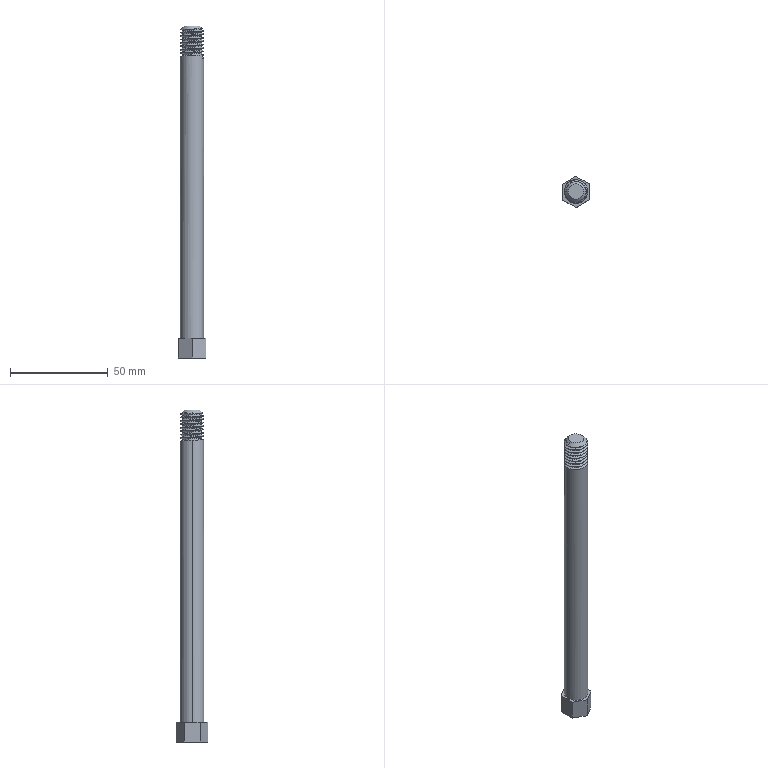Part | SolidWorks | features BaseBody 1 | 1 solid | 32 faces | box 14.038 x 16 x 170 mm | volume 19424 mm3 | cylinder 17 | plane 10 | spline 3 | cone 2 | commonest cylinder face diameters 12 x17